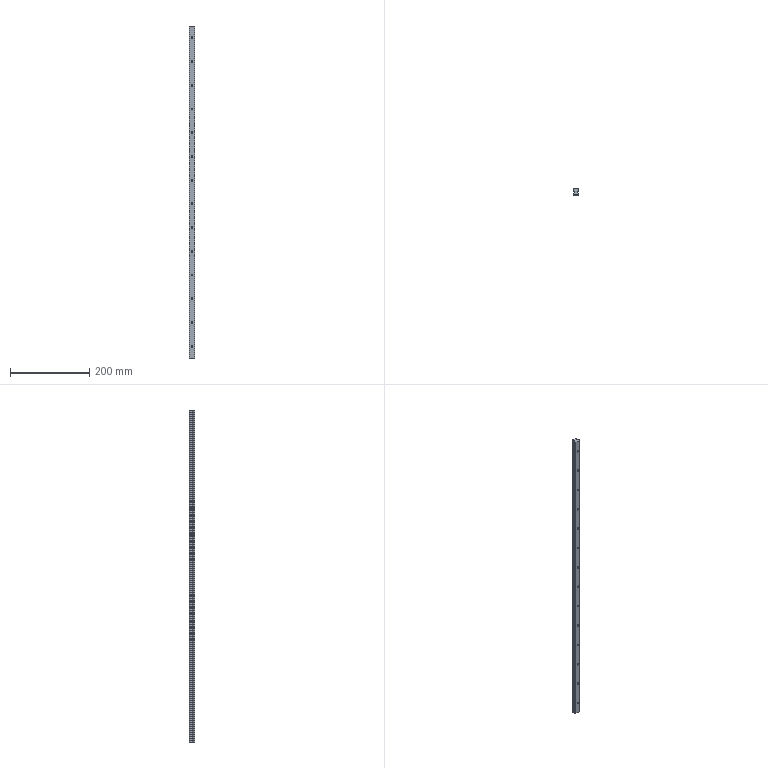Part | SolidWorks | features Extrusion 1, HoleWzd 1, ICE 1, LPattern 1 | 1 solid | 203 faces | box 15 x 15 x 840 mm | volume 154798 mm3 | plane 116 | cylinder 70 | spline 17 | commonest cylinder face diameters 4.5 x28 7.5 x28 0.8 x8 3.24 x4 2 x2